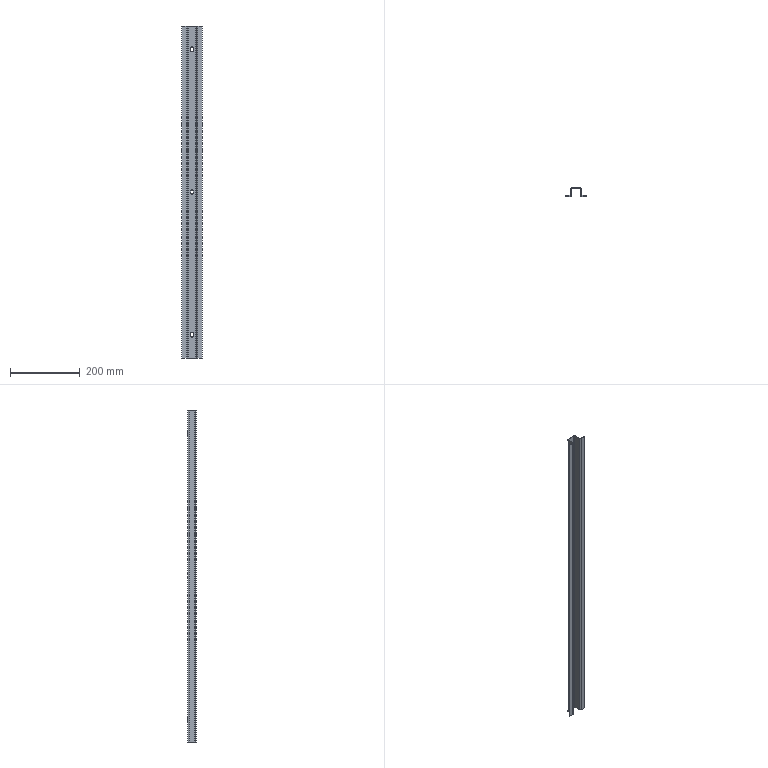Part | STEP file | B_SYL0380DJ1006_2_23-2_STEP | 1 solid | 56 faces | box 60 x 25 x 952 mm | volume 191493 mm3 | plane 36 | cylinder 20 | commonest cylinder face diameters 7 x12 4 x4 8 x4
STEP:
#1=CARTESIAN_POINT('',(-3.5,23.,-405.5));
#2=VERTEX_POINT('',#1);
#3=CARTESIAN_POINT('',(-3.5,25.,-405.5));
#4=VERTEX_POINT('',#3);
#5=CARTESIAN_POINT('',(-3.5,25.,-405.5));
#6=DIRECTION('',(0.,1.,0.));
#7=VECTOR('',#6,1000.);
#8=LINE('',#5,#7);
#9=EDGE_CURVE('',#2,#4,#8,.T.);
#10=ORIENTED_EDGE('',*,*,#9,.F.);
#11=CARTESIAN_POINT('',(-3.5,23.,-412.5));
#12=VERTEX_POINT('',#11);
#13=CARTESIAN_POINT('',(-3.5,23.,-476.));
#14=DIRECTION('',(0.,0.,1.));
#15=VECTOR('',#14,1000.);
#16=LINE('',#13,#15);
#17=EDGE_CURVE('',#12,#2,#16,.T.);
#18=ORIENTED_EDGE('',*,*,#17,.F.);
#19=CARTESIAN_POINT('',(-3.5,25.,-412.5));
#20=VERTEX_POINT('',#19);
#21=CARTESIAN_POINT('',(-3.5,25.,-412.5));
#22=DIRECTION('',(0.,1.,0.));
#23=VECTOR('',#22,1000.);
#24=LINE('',#21,#23);
#25=EDGE_CURVE('',#12,#20,#24,.T.);
#26=ORIENTED_EDGE('',*,*,#25,.T.);
#27=CARTESIAN_POINT('',(-3.5,25.,-412.5));
#28=DIRECTION('',(0.,0.,1.));
#29=VECTOR('',#28,1000.);
#30=LINE('',#27,#29);
#31=EDGE_CURVE('',#20,#4,#30,.T.);
#32=ORIENTED_EDGE('',*,*,#31,.T.);
#33=EDGE_LOOP('',(#10,#18,#26,#32));
#34=FACE_OUTER_BOUND('',#33,.T.);
#35=CARTESIAN_POINT('',(-3.5,25.,-412.5));
#36=DIRECTION('',(1.,0.,0.));
#37=DIRECTION('',(0.,0.,1.));
#38=AXIS2_PLACEMENT_3D('',#35,#36,#37);
#39=PLANE('',#38);
#40=ADVANCED_FACE('',(#34),#39,.T.);
#41=ORIENTED_EDGE('',*,*,#25,.F.);
#42=CARTESIAN_POINT('',(0.,23.,-416.));
#43=VERTEX_POINT('',#42);
#44=CARTESIAN_POINT('',(0.,23.,-412.5));
#45=DIRECTION('',(0.,-1.,0.));
#46=DIRECTION('',(0.,0.,-1.));
#47=AXIS2_PLACEMENT_3D('',#44,#45,#46);
#48=CIRCLE('',#47,3.5);
#49=EDGE_CURVE('',#12,#43,#48,.T.);
#50=ORIENTED_EDGE('',*,*,#49,.T.);
#51=CARTESIAN_POINT('',(0.,25.,-416.));
#52=VERTEX_POINT('',#51);
#53=CARTESIAN_POINT('',(0.,25.,-416.));
#54=DIRECTION('',(0.,1.,0.));
#55=VECTOR('',#54,1000.);
#56=LINE('',#53,#55);
#57=EDGE_CURVE('',#43,#52,#56,.T.);
#58=ORIENTED_EDGE('',*,*,#57,.T.);
#59=CARTESIAN_POINT('',(0.,25.,-412.5));
#60=DIRECTION('',(0.,-1.,0.));
#61=DIRECTION('',(-1.,0.,0.));
#62=AXIS2_PLACEMENT_3D('',#59,#60,#61);
#63=CIRCLE('',#62,3.5);
#64=EDGE_CURVE('',#20,#52,#63,.T.);
#65=ORIENTED_EDGE('',*,*,#64,.F.);
#66=EDGE_LOOP('',(#41,#50,#58,#65));
#67=FACE_OUTER_BOUND('',#66,.T.);
#68=CARTESIAN_POINT('',(0.,25.,-412.5));
#69=DIRECTION('',(0.,-1.,0.));
#70=DIRECTION('',(0.,0.,-1.));
#71=AXIS2_PLACEMENT_3D('',#68,#69,#70);
#72=CYLINDRICAL_SURFACE('',#71,3.5);
#73=ADVANCED_FACE('',(#67),#72,.F.);
#74=ORIENTED_EDGE('',*,*,#57,.F.);
#75=CARTESIAN_POINT('',(3.5,23.,-412.5));
#76=VERTEX_POINT('',#75);
#77=CARTESIAN_POINT('',(0.,23.,-412.5));
#78=DIRECTION('',(0.,-1.,0.));
#79=DIRECTION('',(0.,0.,-1.));
#80=AXIS2_PLACEMENT_3D('',#77,#78,#79);
#81=CIRCLE('',#80,3.5);
#82=EDGE_CURVE('',#43,#76,#81,.T.);
#83=ORIENTED_EDGE('',*,*,#82,.T.);
#84=CARTESIAN_POINT('',(3.5,25.,-412.5));
#85=VERTEX_POINT('',#84);
#86=CARTESIAN_POINT('',(3.5,25.,-412.5));
#87=DIRECTION('',(0.,1.,0.));
#88=VECTOR('',#87,1000.);
#89=LINE('',#86,#88);
#90=EDGE_CURVE('',#76,#85,#89,.T.);
#91=ORIENTED_EDGE('',*,*,#90,.T.);
#92=CARTESIAN_POINT('',(0.,25.,-412.5));
#93=DIRECTION('',(0.,-1.,0.));
#94=DIRECTION('',(0.,0.,-1.));
#95=AXIS2_PLACEMENT_3D('',#92,#93,#94);
#96=CIRCLE('',#95,3.5);
#97=EDGE_CURVE('',#52,#85,#96,.T.);
#98=ORIENTED_EDGE('',*,*,#97,.F.);
#99=EDGE_LOOP('',(#74,#83,#91,#98));
#100=FACE_OUTER_BOUND('',#99,.T.);
#101=CARTESIAN_POINT('',(0.,25.,-412.5));
#102=DIRECTION('',(0.,-1.,0.));
#103=DIRECTION('',(0.,0.,-1.));
#104=AXIS2_PLACEMENT_3D('',#101,#102,#103);
#105=CYLINDRICAL_SURFACE('',#104,3.5);
#106=ADVANCED_FACE('',(#100),#105,.F.);
#107=ORIENTED_EDGE('',*,*,#90,.F.);
#108=CARTESIAN_POINT('',(3.5,23.,-405.5));
#109=VERTEX_POINT('',#108);
#110=CARTESIAN_POINT('',(3.5,23.,-476.));
#111=DIRECTION('',(0.,0.,-1.));
#112=VECTOR('',#111,1000.);
#113=LINE('',#110,#112);
#114=EDGE_CURVE('',#109,#76,#113,.T.);
#115=ORIENTED_EDGE('',*,*,#114,.F.);
#116=CARTESIAN_POINT('',(3.5,25.,-405.5));
#117=VERTEX_POINT('',#116);
#118=CARTESIAN_POINT('',(3.5,25.,-405.5));
#119=DIRECTION('',(0.,1.,0.));
#120=VECTOR('',#119,1000.);
#121=LINE('',#118,#120);
#122=EDGE_CURVE('',#109,#117,#121,.T.);
#123=ORIENTED_EDGE('',*,*,#122,.T.);
#124=CARTESIAN_POINT('',(3.5,25.,-405.5));
#125=DIRECTION('',(0.,0.,-1.));
#126=VECTOR('',#125,1000.);
#127=LINE('',#124,#126);
#128=EDGE_CURVE('',#117,#85,#127,.T.);
#129=ORIENTED_EDGE('',*,*,#128,.T.);
#130=EDGE_LOOP('',(#107,#115,#123,#129));
#131=FACE_OUTER_BOUND('',#130,.T.);
#132=CARTESIAN_POINT('',(3.5,25.,-405.5));
#133=DIRECTION('',(-1.,0.,0.));
#134=DIRECTION('',(0.,0.,-1.));
#135=AXIS2_PLACEMENT_3D('',#132,#133,#134);
#136=PLANE('',#135);
#137=ADVANCED_FACE('',(#131),#136,.T.);
#138=ORIENTED_EDGE('',*,*,#122,.F.);
#139=CARTESIAN_POINT('',(0.,23.,-402.));
#140=VERTEX_POINT('',#139);
#141=CARTESIAN_POINT('',(0.,23.,-405.5));
#142=DIRECTION('',(0.,-1.,0.));
#143=DIRECTION('',(0.,0.,-1.));
#144=AXIS2_PLACEMENT_3D('',#141,#142,#143);
#145=CIRCLE('',#144,3.5);
#146=EDGE_CURVE('',#109,#140,#145,.T.);
#147=ORIENTED_EDGE('',*,*,#146,.T.);
#148=CARTESIAN_POINT('',(0.,25.,-402.));
#149=VERTEX_POINT('',#148);
#150=CARTESIAN_POINT('',(0.,25.,-402.));
#151=DIRECTION('',(0.,1.,0.));
#152=VECTOR('',#151,1000.);
#153=LINE('',#150,#152);
#154=EDGE_CURVE('',#140,#149,#153,.T.);
#155=ORIENTED_EDGE('',*,*,#154,.T.);
#156=CARTESIAN_POINT('',(0.,25.,-405.5));
#157=DIRECTION('',(0.,-1.,0.));
#158=DIRECTION('',(1.,0.,0.));
#159=AXIS2_PLACEMENT_3D('',#156,#157,#158);
#160=CIRCLE('',#159,3.5);
#161=EDGE_CURVE('',#117,#149,#160,.T.);
#162=ORIENTED_EDGE('',*,*,#161,.F.);
#163=EDGE_LOOP('',(#138,#147,#155,#162));
#164=FACE_OUTER_BOUND('',#163,.T.);
#165=CARTESIAN_POINT('',(0.,25.,-405.5));
#166=DIRECTION('',(0.,-1.,0.));
#167=DIRECTION('',(0.,0.,-1.));
#168=AXIS2_PLACEMENT_3D('',#165,#166,#167);
#169=CYLINDRICAL_SURFACE('',#168,3.5);
#170=ADVANCED_FACE('',(#164),#169,.F.);
#171=CARTESIAN_POINT('',(-3.5,23.,3.5));
#172=VERTEX_POINT('',#171);
#173=CARTESIAN_POINT('',(-3.5,25.,3.5));
#174=VERTEX_POINT('',#173);
#175=CARTESIAN_POINT('',(-3.5,25.,3.5));
#176=DIRECTION('',(0.,1.,0.));
#177=VECTOR('',#176,1000.);
#178=LINE('',#175,#177);
#179=EDGE_CURVE('',#172,#174,#178,.T.);
#180=ORIENTED_EDGE('',*,*,#179,.F.);
#181=CARTESIAN_POINT('',(-3.5,23.,-3.5));
#182=VERTEX_POINT('',#181);
#183=CARTESIAN_POINT('',(-3.5,23.,-476.));
#184=DIRECTION('',(0.,0.,1.));
#185=VECTOR('',#184,1000.);
#186=LINE('',#183,#185);
#187=EDGE_CURVE('',#182,#172,#186,.T.);
#188=ORIENTED_EDGE('',*,*,#187,.F.);
#189=CARTESIAN_POINT('',(-3.5,25.,-3.5));
#190=VERTEX_POINT('',#189);
#191=CARTESIAN_POINT('',(-3.5,25.,-3.5));
#192=DIRECTION('',(0.,1.,0.));
#193=VECTOR('',#192,1000.);
#194=LINE('',#191,#193);
#195=EDGE_CURVE('',#182,#190,#194,.T.);
#196=ORIENTED_EDGE('',*,*,#195,.T.);
#197=CARTESIAN_POINT('',(-3.5,25.,-3.5));
#198=DIRECTION('',(0.,0.,1.));
#199=VECTOR('',#198,1000.);
#200=LINE('',#197,#199);
#201=EDGE_CURVE('',#190,#174,#200,.T.);
#202=ORIENTED_EDGE('',*,*,#201,.T.);
#203=EDGE_LOOP('',(#180,#188,#196,#202));
#204=FACE_OUTER_BOUND('',#203,.T.);
#205=CARTESIAN_POINT('',(-3.5,25.,-3.5));
#206=DIRECTION('',(1.,0.,0.));
#207=DIRECTION('',(0.,0.,1.));
#208=AXIS2_PLACEMENT_3D('',#205,#206,#207);
#209=PLANE('',#208);
#210=ADVANCED_FACE('',(#204),#209,.T.);
#211=ORIENTED_EDGE('',*,*,#195,.F.);
#212=CARTESIAN_POINT('',(0.,23.,-7.));
#213=VERTEX_POINT('',#212);
#214=CARTESIAN_POINT('',(0.,23.,-3.5));
#215=DIRECTION('',(0.,-1.,0.));
#216=DIRECTION('',(0.,0.,-1.));
#217=AXIS2_PLACEMENT_3D('',#214,#215,#216);
#218=CIRCLE('',#217,3.5);
#219=EDGE_CURVE('',#182,#213,#218,.T.);
#220=ORIENTED_EDGE('',*,*,#219,.T.);
#221=CARTESIAN_POINT('',(0.,25.,-7.));
#222=VERTEX_POINT('',#221);
#223=CARTESIAN_POINT('',(0.,25.,-7.));
#224=DIRECTION('',(0.,1.,0.));
#225=VECTOR('',#224,1000.);
#226=LINE('',#223,#225);
#227=EDGE_CURVE('',#213,#222,#226,.T.);
#228=ORIENTED_EDGE('',*,*,#227,.T.);
#229=CARTESIAN_POINT('',(0.,25.,-3.5));
#230=DIRECTION('',(0.,-1.,0.));
#231=DIRECTION('',(-1.,0.,0.));
#232=AXIS2_PLACEMENT_3D('',#229,#230,#231);
#233=CIRCLE('',#232,3.5);
#234=EDGE_CURVE('',#190,#222,#233,.T.);
#235=ORIENTED_EDGE('',*,*,#234,.F.);
#236=EDGE_LOOP('',(#211,#220,#228,#235));
#237=FACE_OUTER_BOUND('',#236,.T.);
#238=CARTESIAN_POINT('',(0.,25.,-3.5));
#239=DIRECTION('',(0.,-1.,0.));
#240=DIRECTION('',(0.,0.,-1.));
#241=AXIS2_PLACEMENT_3D('',#238,#239,#240);
#242=CYLINDRICAL_SURFACE('',#241,3.5);
#243=ADVANCED_FACE('',(#237),#242,.F.);
#244=ORIENTED_EDGE('',*,*,#227,.F.);
#245=CARTESIAN_POINT('',(3.5,23.,-3.5));
#246=VERTEX_POINT('',#245);
#247=CARTESIAN_POINT('',(0.,23.,-3.5));
#248=DIRECTION('',(0.,-1.,0.));
#249=DIRECTION('',(0.,0.,-1.));
#250=AXIS2_PLACEMENT_3D('',#247,#248,#249);
#251=CIRCLE('',#250,3.5);
#252=EDGE_CURVE('',#213,#246,#251,.T.);
#253=ORIENTED_EDGE('',*,*,#252,.T.);
#254=CARTESIAN_POINT('',(3.5,25.,-3.5));
#255=VERTEX_POINT('',#254);
#256=CARTESIAN_POINT('',(3.5,25.,-3.5));
#257=DIRECTION('',(0.,1.,0.));
#258=VECTOR('',#257,1000.);
#259=LINE('',#256,#258);
#260=EDGE_CURVE('',#246,#255,#259,.T.);
#261=ORIENTED_EDGE('',*,*,#260,.T.);
#262=CARTESIAN_POINT('',(0.,25.,-3.5));
#263=DIRECTION('',(0.,-1.,0.));
#264=DIRECTION('',(0.,0.,-1.));
#265=AXIS2_PLACEMENT_3D('',#262,#263,#264);
#266=CIRCLE('',#265,3.5);
#267=EDGE_CURVE('',#222,#255,#266,.T.);
#268=ORIENTED_EDGE('',*,*,#267,.F.);
#269=EDGE_LOOP('',(#244,#253,#261,#268));
#270=FACE_OUTER_BOUND('',#269,.T.);
#271=CARTESIAN_POINT('',(0.,25.,-3.5));
#272=DIRECTION('',(0.,-1.,0.));
#273=DIRECTION('',(0.,0.,-1.));
#274=AXIS2_PLACEMENT_3D('',#271,#272,#273);
#275=CYLINDRICAL_SURFACE('',#274,3.5);
#276=ADVANCED_FACE('',(#270),#275,.F.);
#277=ORIENTED_EDGE('',*,*,#260,.F.);
#278=CARTESIAN_POINT('',(3.5,23.,3.5));
#279=VERTEX_POINT('',#278);
#280=CARTESIAN_POINT('',(3.5,23.,-476.));
#281=DIRECTION('',(0.,0.,-1.));
#282=VECTOR('',#281,1000.);
#283=LINE('',#280,#282);
#284=EDGE_CURVE('',#279,#246,#283,.T.);
#285=ORIENTED_EDGE('',*,*,#284,.F.);
#286=CARTESIAN_POINT('',(3.5,25.,3.5));
#287=VERTEX_POINT('',#286);
#288=CARTESIAN_POINT('',(3.5,25.,3.5));
#289=DIRECTION('',(0.,1.,0.));
#290=VECTOR('',#289,1000.);
#291=LINE('',#288,#290);
#292=EDGE_CURVE('',#279,#287,#291,.T.);
#293=ORIENTED_EDGE('',*,*,#292,.T.);
#294=CARTESIAN_POINT('',(3.5,25.,3.5));
#295=DIRECTION('',(0.,0.,-1.));
#296=VECTOR('',#295,1000.);
#297=LINE('',#294,#296);
#298=EDGE_CURVE('',#287,#255,#297,.T.);
#299=ORIENTED_EDGE('',*,*,#298,.T.);
#300=EDGE_LOOP('',(#277,#285,#293,#299));
#301=FACE_OUTER_BOUND('',#300,.T.);
#302=CARTESIAN_POINT('',(3.5,25.,3.5));
#303=DIRECTION('',(-1.,0.,0.));
#304=DIRECTION('',(0.,0.,-1.));
#305=AXIS2_PLACEMENT_3D('',#302,#303,#304);
#306=PLANE('',#305);
#307=ADVANCED_FACE('',(#301),#306,.T.);
#308=ORIENTED_EDGE('',*,*,#292,.F.);
#309=CARTESIAN_POINT('',(0.,23.,7.));
#310=VERTEX_POINT('',#309);
#311=CARTESIAN_POINT('',(0.,23.,3.5));
#312=DIRECTION('',(0.,-1.,0.));
#313=DIRECTION('',(0.,0.,-1.));
#314=AXIS2_PLACEMENT_3D('',#311,#312,#313);
#315=CIRCLE('',#314,3.5);
#316=EDGE_CURVE('',#279,#310,#315,.T.);
#317=ORIENTED_EDGE('',*,*,#316,.T.);
#318=CARTESIAN_POINT('',(0.,25.,7.));
#319=VERTEX_POINT('',#318);
#320=CARTESIAN_POINT('',(0.,25.,7.));
#321=DIRECTION('',(0.,1.,0.));
#322=VECTOR('',#321,1000.);
#323=LINE('',#320,#322);
#324=EDGE_CURVE('',#310,#319,#323,.T.);
#325=ORIENTED_EDGE('',*,*,#324,.T.);
#326=CARTESIAN_POINT('',(0.,25.,3.5));
#327=DIRECTION('',(0.,-1.,0.));
#328=DIRECTION('',(1.,0.,0.));
#329=AXIS2_PLACEMENT_3D('',#326,#327,#328);
#330=CIRCLE('',#329,3.5);
#331=EDGE_CURVE('',#287,#319,#330,.T.);
#332=ORIENTED_EDGE('',*,*,#331,.F.);
#333=EDGE_LOOP('',(#308,#317,#325,#332));
#334=FACE_OUTER_BOUND('',#333,.T.);
#335=CARTESIAN_POINT('',(0.,25.,3.5));
#336=DIRECTION('',(0.,-1.,0.));
#337=DIRECTION('',(0.,0.,-1.));
#338=AXIS2_PLACEMENT_3D('',#335,#336,#337);
#339=CYLINDRICAL_SURFACE('',#338,3.5);
#340=ADVANCED_FACE('',(#334),#339,.F.);
#341=CARTESIAN_POINT('',(-3.5,23.,412.5));
#342=VERTEX_POINT('',#341);
#343=CARTESIAN_POINT('',(-3.5,25.,412.5));
#344=VERTEX_POINT('',#343);
#345=CARTESIAN_POINT('',(-3.5,25.,412.5));
#346=DIRECTION('',(0.,1.,0.));
#347=VECTOR('',#346,1000.);
#348=LINE('',#345,#347);
#349=EDGE_CURVE('',#342,#344,#348,.T.);
#350=ORIENTED_EDGE('',*,*,#349,.F.);
#351=CARTESIAN_POINT('',(-3.5,23.,405.5));
#352=VERTEX_POINT('',#351);
#353=CARTESIAN_POINT('',(-3.5,23.,-476.));
#354=DIRECTION('',(0.,0.,1.));
#355=VECTOR('',#354,1000.);
#356=LINE('',#353,#355);
#357=EDGE_CURVE('',#352,#342,#356,.T.);
#358=ORIENTED_EDGE('',*,*,#357,.F.);
#359=CARTESIAN_POINT('',(-3.5,25.,405.5));
#360=VERTEX_POINT('',#359);
#361=CARTESIAN_POINT('',(-3.5,25.,405.5));
#362=DIRECTION('',(0.,1.,0.));
#363=VECTOR('',#362,1000.);
#364=LINE('',#361,#363);
#365=EDGE_CURVE('',#352,#360,#364,.T.);
#366=ORIENTED_EDGE('',*,*,#365,.T.);
#367=CARTESIAN_POINT('',(-3.5,25.,405.5));
#368=DIRECTION('',(0.,0.,1.));
#369=VECTOR('',#368,1000.);
#370=LINE('',#367,#369);
#371=EDGE_CURVE('',#360,#344,#370,.T.);
#372=ORIENTED_EDGE('',*,*,#371,.T.);
#373=EDGE_LOOP('',(#350,#358,#366,#372));
#374=FACE_OUTER_BOUND('',#373,.T.);
#375=CARTESIAN_POINT('',(-3.5,25.,405.5));
#376=DIRECTION('',(1.,0.,0.));
#377=DIRECTION('',(0.,0.,1.));
#378=AXIS2_PLACEMENT_3D('',#375,#376,#377);
#379=PLANE('',#378);
#380=ADVANCED_FACE('',(#374),#379,.T.);
#381=ORIENTED_EDGE('',*,*,#365,.F.);
#382=CARTESIAN_POINT('',(0.,23.,402.));
#383=VERTEX_POINT('',#382);
#384=CARTESIAN_POINT('',(0.,23.,405.5));
#385=DIRECTION('',(0.,-1.,0.));
#386=DIRECTION('',(0.,0.,-1.));
#387=AXIS2_PLACEMENT_3D('',#384,#385,#386);
#388=CIRCLE('',#387,3.5);
#389=EDGE_CURVE('',#352,#383,#388,.T.);
#390=ORIENTED_EDGE('',*,*,#389,.T.);
#391=CARTESIAN_POINT('',(0.,25.,402.));
#392=VERTEX_POINT('',#391);
#393=CARTESIAN_POINT('',(0.,25.,402.));
#394=DIRECTION('',(0.,1.,0.));
#395=VECTOR('',#394,1000.);
#396=LINE('',#393,#395);
#397=EDGE_CURVE('',#383,#392,#396,.T.);
#398=ORIENTED_EDGE('',*,*,#397,.T.);
#399=CARTESIAN_POINT('',(0.,25.,405.5));
#400=DIRECTION('',(0.,-1.,0.));
#401=DIRECTION('',(-1.,0.,0.));
#402=AXIS2_PLACEMENT_3D('',#399,#400,#401);
#403=CIRCLE('',#402,3.5);
#404=EDGE_CURVE('',#360,#392,#403,.T.);
#405=ORIENTED_EDGE('',*,*,#404,.F.);
#406=EDGE_LOOP('',(#381,#390,#398,#405));
#407=FACE_OUTER_BOUND('',#406,.T.);
#408=CARTESIAN_POINT('',(0.,25.,405.5));
#409=DIRECTION('',(0.,-1.,0.));
#410=DIRECTION('',(0.,0.,-1.));
#411=AXIS2_PLACEMENT_3D('',#408,#409,#410);
#412=CYLINDRICAL_SURFACE('',#411,3.5);
#413=ADVANCED_FACE('',(#407),#412,.F.);
#414=ORIENTED_EDGE('',*,*,#397,.F.);
#415=CARTESIAN_POINT('',(3.5,23.,405.5));
#416=VERTEX_POINT('',#415);
#417=CARTESIAN_POINT('',(0.,23.,405.5));
#418=DIRECTION('',(0.,-1.,0.));
#419=DIRECTION('',(0.,0.,-1.));
#420=AXIS2_PLACEMENT_3D('',#417,#418,#419);
#421=CIRCLE('',#420,3.5);
#422=EDGE_CURVE('',#383,#416,#421,.T.);
#423=ORIENTED_EDGE('',*,*,#422,.T.);
#424=CARTESIAN_POINT('',(3.5,25.,405.5));
#425=VERTEX_POINT('',#424);
#426=CARTESIAN_POINT('',(3.5,25.,405.5));
#427=DIRECTION('',(0.,1.,0.));
#428=VECTOR('',#427,1000.);
#429=LINE('',#426,#428);
#430=EDGE_CURVE('',#416,#425,#429,.T.);
#431=ORIENTED_EDGE('',*,*,#430,.T.);
#432=CARTESIAN_POINT('',(0.,25.,405.5));
#433=DIRECTION('',(0.,-1.,0.));
#434=DIRECTION('',(0.,0.,-1.));
#435=AXIS2_PLACEMENT_3D('',#432,#433,#434);
#436=CIRCLE('',#435,3.5);
#437=EDGE_CURVE('',#392,#425,#436,.T.);
#438=ORIENTED_EDGE('',*,*,#437,.F.);
#439=EDGE_LOOP('',(#414,#423,#431,#438));
#440=FACE_OUTER_BOUND('',#439,.T.);
#441=CARTESIAN_POINT('',(0.,25.,405.5));
#442=DIRECTION('',(0.,-1.,0.));
#443=DIRECTION('',(0.,0.,-1.));
#444=AXIS2_PLACEMENT_3D('',#441,#442,#443);
#445=CYLINDRICAL_SURFACE('',#444,3.5);
#446=ADVANCED_FACE('',(#440),#445,.F.);
#447=ORIENTED_EDGE('',*,*,#430,.F.);
#448=CARTESIAN_POINT('',(3.5,23.,412.5));
#449=VERTEX_POINT('',#448);
#450=CARTESIAN_POINT('',(3.5,23.,-476.));
#451=DIRECTION('',(0.,0.,-1.));
#452=VECTOR('',#451,1000.);
#453=LINE('',#450,#452);
#454=EDGE_CURVE('',#449,#416,#453,.T.);
#455=ORIENTED_EDGE('',*,*,#454,.F.);
#456=CARTESIAN_POINT('',(3.5,25.,412.5));
#457=VERTEX_POINT('',#456);
#458=CARTESIAN_POINT('',(3.5,25.,412.5));
#459=DIRECTION('',(0.,1.,0.));
#460=VECTOR('',#459,1000.);
#461=LINE('',#458,#460);
#462=EDGE_CURVE('',#449,#457,#461,.T.);
#463=ORIENTED_EDGE('',*,*,#462,.T.);
#464=CARTESIAN_POINT('',(3.5,25.,412.5));
#465=DIRECTION('',(0.,0.,-1.));
#466=VECTOR('',#465,1000.);
#467=LINE('',#464,#466);
#468=EDGE_CURVE('',#457,#425,#467,.T.);
#469=ORIENTED_EDGE('',*,*,#468,.T.);
#470=EDGE_LOOP('',(#447,#455,#463,#469));
#471=FACE_OUTER_BOUND('',#470,.T.);
#472=CARTESIAN_POINT('',(3.5,25.,412.5));
#473=DIRECTION('',(-1.,0.,0.));
#474=DIRECTION('',(0.,0.,-1.));
#475=AXIS2_PLACEMENT_3D('',#472,#473,#474);
#476=PLANE('',#475);
#477=ADVANCED_FACE('',(#471),#476,.T.);
#478=ORIENTED_EDGE('',*,*,#462,.F.);
#479=CARTESIAN_POINT('',(0.,23.,416.));
#480=VERTEX_POINT('',#479);
#481=CARTESIAN_POINT('',(0.,23.,412.5));
#482=DIRECTION('',(0.,-1.,0.));
#483=DIRECTION('',(0.,0.,-1.));
#484=AXIS2_PLACEMENT_3D('',#481,#482,#483);
#485=CIRCLE('',#484,3.5);
#486=EDGE_CURVE('',#449,#480,#485,.T.);
#487=ORIENTED_EDGE('',*,*,#486,.T.);
#488=CARTESIAN_POINT('',(0.,25.,416.));
#489=VERTEX_POINT('',#488);
#490=CARTESIAN_POINT('',(0.,25.,416.));
#491=DIRECTION('',(0.,1.,0.));
#492=VECTOR('',#491,1000.);
#493=LINE('',#490,#492);
#494=EDGE_CURVE('',#480,#489,#493,.T.);
#495=ORIENTED_EDGE('',*,*,#494,.T.);
#496=CARTESIAN_POINT('',(0.,25.,412.5));
#497=DIRECTION('',(0.,-1.,0.));
#498=DIRECTION('',(1.,0.,0.));
#499=AXIS2_PLACEMENT_3D('',#496,#497,#498);
#500=CIRCLE('',#499,3.5);
#501=EDGE_CURVE('',#457,#489,#500,.T.);
#502=ORIENTED_EDGE('',*,*,#501,.F.);
#503=EDGE_LOOP('',(#478,#487,#495,#502));
#504=FACE_OUTER_BOUND('',#503,.T.);
#505=CARTESIAN_POINT('',(0.,25.,412.5));
#506=DIRECTION('',(0.,-1.,0.));
#507=DIRECTION('',(0.,0.,-1.));
#508=AXIS2_PLACEMENT_3D('',#505,#506,#507);
#509=CYLINDRICAL_SURFACE('',#508,3.5);
#510=ADVANCED_FACE('',(#504),#509,.F.);
#511=CARTESIAN_POINT('',(-30.,0.,-476.));
#512=VERTEX_POINT('',#511);
#513=CARTESIAN_POINT('',(-30.,2.,-476.));
#514=VERTEX_POINT('',#513);
#515=CARTESIAN_POINT('',(-30.,2.,-476.));
#516=DIRECTION('',(0.,1.,0.));
#517=VECTOR('',#516,1000.);
#518=LINE('',#515,#517);
#519=EDGE_CURVE('',#512,#514,#518,.T.);
#520=ORIENTED_EDGE('',*,*,#519,.F.);
#521=CARTESIAN_POINT('',(-30.,0.,476.));
#522=VERTEX_POINT('',#521);
#523=CARTESIAN_POINT('',(-30.,0.,-476.));
#524=DIRECTION('',(0.,0.,-1.));
#525=VECTOR('',#524,1000.);
#526=LINE('',#523,#525);
#527=EDGE_CURVE('',#522,#512,#526,.T.);
#528=ORIENTED_EDGE('',*,*,#527,.F.);
#529=CARTESIAN_POINT('',(-30.,2.,476.));
#530=VERTEX_POINT('',#529);
#531=CARTESIAN_POINT('',(-30.,2.,476.));
#532=DIRECTION('',(0.,1.,0.));
#533=VECTOR('',#532,1000.);
#534=LINE('',#531,#533);
#535=EDGE_CURVE('',#522,#530,#534,.T.);
#536=ORIENTED_EDGE('',*,*,#535,.T.);
#537=CARTESIAN_POINT('',(-30.,2.,476.));
#538=DIRECTION('',(0.,0.,-1.));
#539=VECTOR('',#538,1000.);
#540=LINE('',#537,#539);
#541=EDGE_CURVE('',#530,#514,#540,.T.);
#542=ORIENTED_EDGE('',*,*,#541,.T.);
#543=EDGE_LOOP('',(#520,#528,#536,#542));
#544=FACE_OUTER_BOUND('',#543,.T.);
#545=CARTESIAN_POINT('',(-30.,2.,476.));
#546=DIRECTION('',(-1.,0.,0.));
#547=DIRECTION('',(0.,0.,-1.));
#548=AXIS2_PLACEMENT_3D('',#545,#546,#547);
#549=PLANE('',#548);
#550=ADVANCED_FACE('',(#544),#549,.T.);
#551=ORIENTED_EDGE('',*,*,#535,.F.);
#552=CARTESIAN_POINT('',(-17.,0.,476.));
#553=VERTEX_POINT('',#552);
#554=CARTESIAN_POINT('',(-30.,0.,476.));
#555=DIRECTION('',(-1.,0.,0.));
#556=VECTOR('',#555,1000.);
#557=LINE('',#554,#556);
#558=EDGE_CURVE('',#553,#522,#557,.T.);
#559=ORIENTED_EDGE('',*,*,#558,.F.);
#560=CARTESIAN_POINT('',(-17.,2.,476.));
#561=VERTEX_POINT('',#560);
#562=CARTESIAN_POINT('',(-17.,2.,476.));
#563=DIRECTION('',(0.,1.,0.));
#564=VECTOR('',#563,1000.);
#565=LINE('',#562,#564);
#566=EDGE_CURVE('',#553,#561,#565,.T.);
#567=ORIENTED_EDGE('',*,*,#566,.T.);
#568=CARTESIAN_POINT('',(-17.,2.,476.));
#569=DIRECTION('',(-1.,0.,0.));
#570=VECTOR('',#569,1000.);
#571=LINE('',#568,#570);
#572=EDGE_CURVE('',#561,#530,#571,.T.);
#573=ORIENTED_EDGE('',*,*,#572,.T.);
#574=EDGE_LOOP('',(#551,#559,#567,#573));
#575=FACE_OUTER_BOUND('',#574,.T.);
#576=CARTESIAN_POINT('',(-17.,2.,476.));
#577=DIRECTION('',(0.,0.,1.));
#578=DIRECTION('',(-1.,0.,0.));
#579=AXIS2_PLACEMENT_3D('',#576,#577,#578);
#580=PLANE('',#579);
#581=ADVANCED_FACE('',(#575),#580,.T.);
#582=ORIENTED_EDGE('',*,*,#566,.F.);
#583=CARTESIAN_POINT('',(-13.,4.,476.));
#584=VERTEX_POINT('',#583);
#585=CARTESIAN_POINT('',(-17.,4.,476.));
#586=DIRECTION('',(0.,0.,-1.));
#587=DIRECTION('',(1.,0.,0.));
#588=AXIS2_PLACEMENT_3D('',#585,#586,#587);
#589=CIRCLE('',#588,4.);
#590=EDGE_CURVE('',#584,#553,#589,.T.);
#591=ORIENTED_EDGE('',*,*,#590,.F.);
#592=CARTESIAN_POINT('',(-15.,4.,476.));
#593=VERTEX_POINT('',#592);
#594=CARTESIAN_POINT('',(-15.,4.,476.));
#595=DIRECTION('',(-1.,0.,0.));
#596=VECTOR('',#595,1000.);
#597=LINE('',#594,#596);
#598=EDGE_CURVE('',#584,#593,#597,.T.);
#599=ORIENTED_EDGE('',*,*,#598,.T.);
#600=CARTESIAN_POINT('',(-17.,4.,476.));
#601=DIRECTION('',(0.,0.,-1.));
#602=DIRECTION('',(1.,0.,0.));
#603=AXIS2_PLACEMENT_3D('',#600,#601,#602);
#604=CIRCLE('',#603,2.);
#605=EDGE_CURVE('',#593,#561,#604,.T.);
#606=ORIENTED_EDGE('',*,*,#605,.T.);
#607=EDGE_LOOP('',(#582,#591,#599,#606));
#608=FACE_OUTER_BOUND('',#607,.T.);
#609=CARTESIAN_POINT('',(-17.,4.,476.));
#610=DIRECTION('',(0.,0.,1.));
#611=DIRECTION('',(1.,0.,0.));
#612=AXIS2_PLACEMENT_3D('',#609,#610,#611);
#613=PLANE('',#612);
#614=ADVANCED_FACE('',(#608),#613,.T.);
#615=ORIENTED_EDGE('',*,*,#598,.F.);
#616=CARTESIAN_POINT('',(-13.,21.,476.));
#617=VERTEX_POINT('',#616);
#618=CARTESIAN_POINT('',(-13.,4.,476.));
#619=DIRECTION('',(0.,-1.,0.));
#620=VECTOR('',#619,1000.);
#621=LINE('',#618,#620);
#622=EDGE_CURVE('',#617,#584,#621,.T.);
#623=ORIENTED_EDGE('',*,*,#622,.F.);
#624=CARTESIAN_POINT('',(-15.,21.,476.));
#625=VERTEX_POINT('',#624);
#626=CARTESIAN_POINT('',(-15.,21.,476.));
#627=DIRECTION('',(-1.,0.,0.));
#628=VECTOR('',#627,1000.);
#629=LINE('',#626,#628);
#630=EDGE_CURVE('',#617,#625,#629,.T.);
#631=ORIENTED_EDGE('',*,*,#630,.T.);
#632=CARTESIAN_POINT('',(-15.,21.,476.));
#633=DIRECTION('',(0.,-1.,0.));
#634=VECTOR('',#633,1000.);
#635=LINE('',#632,#634);
#636=EDGE_CURVE('',#625,#593,#635,.T.);
#637=ORIENTED_EDGE('',*,*,#636,.T.);
#638=EDGE_LOOP('',(#615,#623,#631,#637));
#639=FACE_OUTER_BOUND('',#638,.T.);
#640=CARTESIAN_POINT('',(-15.,21.,476.));
#641=DIRECTION('',(0.,0.,1.));
#642=DIRECTION('',(0.,-1.,0.));
#643=AXIS2_PLACEMENT_3D('',#640,#641,#642);
#644=PLANE('',#643);
#645=ADVANCED_FACE('',(#639),#644,.T.);
#646=ORIENTED_EDGE('',*,*,#630,.F.);
#647=CARTESIAN_POINT('',(-11.,23.,476.));
#648=VERTEX_POINT('',#647);
#649=CARTESIAN_POINT('',(-11.,21.,476.));
#650=DIRECTION('',(0.,0.,1.));
#651=DIRECTION('',(1.,0.,0.));
#652=AXIS2_PLACEMENT_3D('',#649,#650,#651);
#653=CIRCLE('',#652,2.);
#654=EDGE_CURVE('',#648,#617,#653,.T.);
#655=ORIENTED_EDGE('',*,*,#654,.F.);
#656=CARTESIAN_POINT('',(-11.,25.,476.));
#657=VERTEX_POINT('',#656);
#658=CARTESIAN_POINT('',(-11.,25.,476.));
#659=DIRECTION('',(0.,1.,0.));
#660=VECTOR('',#659,1000.);
#661=LINE('',#658,#660);
#662=EDGE_CURVE('',#648,#657,#661,.T.);
#663=ORIENTED_EDGE('',*,*,#662,.T.);
#664=CARTESIAN_POINT('',(-11.,21.,476.));
#665=DIRECTION('',(0.,0.,1.));
#666=DIRECTION('',(0.,1.,0.));
#667=AXIS2_PLACEMENT_3D('',#664,#665,#666);
#668=CIRCLE('',#667,4.);
#669=EDGE_CURVE('',#657,#625,#668,.T.);
#670=ORIENTED_EDGE('',*,*,#669,.T.);
#671=EDGE_LOOP('',(#646,#655,#663,#670));
#672=FACE_OUTER_BOUND('',#671,.T.);
#673=CARTESIAN_POINT('',(-11.,21.,476.));
#674=DIRECTION('',(0.,0.,-1.));
#675=DIRECTION('',(-1.,0.,0.));
#676=AXIS2_PLACEMENT_3D('',#673,#674,#675);
#677=PLANE('',#676);
#678=ADVANCED_FACE('',(#672),#677,.F.);
#679=ORIENTED_EDGE('',*,*,#662,.F.);
#680=CARTESIAN_POINT('',(11.,23.,476.));
#681=VERTEX_POINT('',#680);
#682=CARTESIAN_POINT('',(-11.,23.,476.));
#683=DIRECTION('',(-1.,0.,0.));
#684=VECTOR('',#683,1000.);
#685=LINE('',#682,#684);
#686=EDGE_CURVE('',#681,#648,#685,.T.);
#687=ORIENTED_EDGE('',*,*,#686,.F.);
#688=CARTESIAN_POINT('',(11.,25.,476.));
#689=VERTEX_POINT('',#688);
#690=CARTESIAN_POINT('',(11.,25.,476.));
#691=DIRECTION('',(0.,1.,0.));
#692=VECTOR('',#691,1000.);
#693=LINE('',#690,#692);
#694=EDGE_CURVE('',#681,#689,#693,.T.);
#695=ORIENTED_EDGE('',*,*,#694,.T.);
#696=CARTESIAN_POINT('',(11.,25.,476.));
#697=DIRECTION('',(-1.,0.,0.));
#698=VECTOR('',#697,1000.);
#699=LINE('',#696,#698);
#700=EDGE_CURVE('',#689,#657,#699,.T.);
#701=ORIENTED_EDGE('',*,*,#700,.T.);
#702=EDGE_LOOP('',(#679,#687,#695,#701));
#703=FACE_OUTER_BOUND('',#702,.T.);
#704=CARTESIAN_POINT('',(11.,25.,476.));
#705=DIRECTION('',(0.,0.,1.));
#706=DIRECTION('',(-1.,0.,0.));
#707=AXIS2_PLACEMENT_3D('',#704,#705,#706);
#708=PLANE('',#707);
#709=ADVANCED_FACE('',(#703),#708,.T.);
#710=ORIENTED_EDGE('',*,*,#694,.F.);
#711=CARTESIAN_POINT('',(13.,21.,476.));
#712=VERTEX_POINT('',#711);
#713=CARTESIAN_POINT('',(11.,21.,476.));
#714=DIRECTION('',(0.,0.,1.));
#715=DIRECTION('',(1.,0.,0.));
#716=AXIS2_PLACEMENT_3D('',#713,#714,#715);
#717=CIRCLE('',#716,2.);
#718=EDGE_CURVE('',#712,#681,#717,.T.);
#719=ORIENTED_EDGE('',*,*,#718,.F.);
#720=CARTESIAN_POINT('',(15.,21.,476.));
#721=VERTEX_POINT('',#720);
#722=CARTESIAN_POINT('',(15.,21.,476.));
#723=DIRECTION('',(1.,0.,0.));
#724=VECTOR('',#723,1000.);
#725=LINE('',#722,#724);
#726=EDGE_CURVE('',#712,#721,#725,.T.);
#727=ORIENTED_EDGE('',*,*,#726,.T.);
#728=CARTESIAN_POINT('',(11.,21.,476.));
#729=DIRECTION('',(0.,0.,1.));
#730=DIRECTION('',(1.,0.,0.));
#731=AXIS2_PLACEMENT_3D('',#728,#729,#730);
#732=CIRCLE('',#731,4.);
#733=EDGE_CURVE('',#721,#689,#732,.T.);
#734=ORIENTED_EDGE('',*,*,#733,.T.);
#735=EDGE_LOOP('',(#710,#719,#727,#734));
#736=FACE_OUTER_BOUND('',#735,.T.);
#737=CARTESIAN_POINT('',(11.,21.,476.));
#738=DIRECTION('',(0.,0.,-1.));
#739=DIRECTION('',(-1.,0.,0.));
#740=AXIS2_PLACEMENT_3D('',#737,#738,#739);
#741=PLANE('',#740);
#742=ADVANCED_FACE('',(#736),#741,.F.);
#743=ORIENTED_EDGE('',*,*,#726,.F.);
#744=CARTESIAN_POINT('',(13.,4.,476.));
#745=VERTEX_POINT('',#744);
#746=CARTESIAN_POINT('',(13.,21.,476.));
#747=DIRECTION('',(0.,1.,0.));
#748=VECTOR('',#747,1000.);
#749=LINE('',#746,#748);
#750=EDGE_CURVE('',#745,#712,#749,.T.);
#751=ORIENTED_EDGE('',*,*,#750,.F.);
#752=CARTESIAN_POINT('',(15.,4.,476.));
#753=VERTEX_POINT('',#752);
#754=CARTESIAN_POINT('',(15.,4.,476.));
#755=DIRECTION('',(1.,0.,0.));
#756=VECTOR('',#755,1000.);
#757=LINE('',#754,#756);
#758=EDGE_CURVE('',#745,#753,#757,.T.);
#759=ORIENTED_EDGE('',*,*,#758,.T.);
#760=CARTESIAN_POINT('',(15.,4.,476.));
#761=DIRECTION('',(0.,1.,0.));
#762=VECTOR('',#761,1000.);
#763=LINE('',#760,#762);
#764=EDGE_CURVE('',#753,#721,#763,.T.);
#765=ORIENTED_EDGE('',*,*,#764,.T.);
#766=EDGE_LOOP('',(#743,#751,#759,#765));
#767=FACE_OUTER_BOUND('',#766,.T.);
#768=CARTESIAN_POINT('',(15.,4.,476.));
#769=DIRECTION('',(0.,0.,1.));
#770=DIRECTION('',(0.,1.,0.));
#771=AXIS2_PLACEMENT_3D('',#768,#769,#770);
#772=PLANE('',#771);
#773=ADVANCED_FACE('',(#767),#772,.T.);
#774=ORIENTED_EDGE('',*,*,#758,.F.);
#775=CARTESIAN_POINT('',(17.,0.,476.));
#776=VERTEX_POINT('',#775);
#777=CARTESIAN_POINT('',(17.,4.,476.));
#778=DIRECTION('',(0.,0.,-1.));
#779=DIRECTION('',(1.,0.,0.));
#780=AXIS2_PLACEMENT_3D('',#777,#778,#779);
#781=CIRCLE('',#780,4.);
#782=EDGE_CURVE('',#776,#745,#781,.T.);
#783=ORIENTED_EDGE('',*,*,#782,.F.);
#784=CARTESIAN_POINT('',(17.,2.,476.));
#785=VERTEX_POINT('',#784);
#786=CARTESIAN_POINT('',(17.,2.,476.));
#787=DIRECTION('',(0.,1.,0.));
#788=VECTOR('',#787,1000.);
#789=LINE('',#786,#788);
#790=EDGE_CURVE('',#776,#785,#789,.T.);
#791=ORIENTED_EDGE('',*,*,#790,.T.);
#792=CARTESIAN_POINT('',(17.,4.,476.));
#793=DIRECTION('',(0.,0.,-1.));
#794=DIRECTION('',(0.,-1.,0.));
#795=AXIS2_PLACEMENT_3D('',#792,#793,#794);
#796=CIRCLE('',#795,2.);
#797=EDGE_CURVE('',#785,#753,#796,.T.);
#798=ORIENTED_EDGE('',*,*,#797,.T.);
#799=EDGE_LOOP('',(#774,#783,#791,#798));
#800=FACE_OUTER_BOUND('',#799,.T.);
#801=CARTESIAN_POINT('',(17.,4.,476.));
#802=DIRECTION('',(0.,0.,1.));
#803=DIRECTION('',(1.,0.,0.));
#804=AXIS2_PLACEMENT_3D('',#801,#802,#803);
#805=PLANE('',#804);
#806=ADVANCED_FACE('',(#800),#805,.T.);
#807=ORIENTED_EDGE('',*,*,#790,.F.);
#808=CARTESIAN_POINT('',(30.,0.,476.));
#809=VERTEX_POINT('',#808);
#810=CARTESIAN_POINT('',(17.,0.,476.));
#811=DIRECTION('',(-1.,0.,0.));
#812=VECTOR('',#811,1000.);
#813=LINE('',#810,#812);
#814=EDGE_CURVE('',#809,#776,#813,.T.);
#815=ORIENTED_EDGE('',*,*,#814,.F.);
#816=CARTESIAN_POINT('',(30.,2.,476.));
#817=VERTEX_POINT('',#816);
#818=CARTESIAN_POINT('',(30.,2.,476.));
#819=DIRECTION('',(0.,1.,0.));
#820=VECTOR('',#819,1000.);
#821=LINE('',#818,#820);
#822=EDGE_CURVE('',#809,#817,#821,.T.);
#823=ORIENTED_EDGE('',*,*,#822,.T.);
#824=CARTESIAN_POINT('',(30.,2.,476.));
#825=DIRECTION('',(-1.,0.,0.));
#826=VECTOR('',#825,1000.);
#827=LINE('',#824,#826);
#828=EDGE_CURVE('',#817,#785,#827,.T.);
#829=ORIENTED_EDGE('',*,*,#828,.T.);
#830=EDGE_LOOP('',(#807,#815,#823,#829));
#831=FACE_OUTER_BOUND('',#830,.T.);
#832=CARTESIAN_POINT('',(30.,2.,476.));
#833=DIRECTION('',(0.,0.,1.));
#834=DIRECTION('',(-1.,0.,0.));
#835=AXIS2_PLACEMENT_3D('',#832,#833,#834);
#836=PLANE('',#835);
#837=ADVANCED_FACE('',(#831),#836,.T.);
#838=ORIENTED_EDGE('',*,*,#822,.F.);
#839=CARTESIAN_POINT('',(30.,0.,-476.));
#840=VERTEX_POINT('',#839);
#841=CARTESIAN_POINT('',(30.,0.,-476.));
#842=DIRECTION('',(0.,0.,-1.));
#843=VECTOR('',#842,1000.);
#844=LINE('',#841,#843);
#845=EDGE_CURVE('',#809,#840,#844,.T.);
#846=ORIENTED_EDGE('',*,*,#845,.T.);
#847=CARTESIAN_POINT('',(30.,2.,-476.));
#848=VERTEX_POINT('',#847);
#849=CARTESIAN_POINT('',(30.,2.,-476.));
#850=DIRECTION('',(0.,1.,0.));
#851=VECTOR('',#850,1000.);
#852=LINE('',#849,#851);
#853=EDGE_CURVE('',#840,#848,#852,.T.);
#854=ORIENTED_EDGE('',*,*,#853,.T.);
#855=CARTESIAN_POINT('',(30.,2.,476.));
#856=DIRECTION('',(0.,0.,-1.));
#857=VECTOR('',#856,1000.);
#858=LINE('',#855,#857);
#859=EDGE_CURVE('',#817,#848,#858,.T.);
#860=ORIENTED_EDGE('',*,*,#859,.F.);
#861=EDGE_LOOP('',(#838,#846,#854,#860));
#862=FACE_OUTER_BOUND('',#861,.T.);
#863=CARTESIAN_POINT('',(30.,2.,476.));
#864=DIRECTION('',(-1.,0.,0.));
#865=DIRECTION('',(0.,0.,-1.));
#866=AXIS2_PLACEMENT_3D('',#863,#864,#865);
#867=PLANE('',#866);
#868=ADVANCED_FACE('',(#862),#867,.F.);
#869=ORIENTED_EDGE('',*,*,#853,.F.);
#870=CARTESIAN_POINT('',(17.,0.,-476.));
#871=VERTEX_POINT('',#870);
#872=CARTESIAN_POINT('',(17.,0.,-476.));
#873=DIRECTION('',(-1.,0.,0.));
#874=VECTOR('',#873,1000.);
#875=LINE('',#872,#874);
#876=EDGE_CURVE('',#840,#871,#875,.T.);
#877=ORIENTED_EDGE('',*,*,#876,.T.);
#878=CARTESIAN_POINT('',(17.,2.,-476.));
#879=VERTEX_POINT('',#878);
#880=CARTESIAN_POINT('',(17.,2.,-476.));
#881=DIRECTION('',(0.,1.,0.));
#882=VECTOR('',#881,1000.);
#883=LINE('',#880,#882);
#884=EDGE_CURVE('',#871,#879,#883,.T.);
#885=ORIENTED_EDGE('',*,*,#884,.T.);
#886=CARTESIAN_POINT('',(30.,2.,-476.));
#887=DIRECTION('',(-1.,0.,0.));
#888=VECTOR('',#887,1000.);
#889=LINE('',#886,#888);
#890=EDGE_CURVE('',#848,#879,#889,.T.);
#891=ORIENTED_EDGE('',*,*,#890,.F.);
#892=EDGE_LOOP('',(#869,#877,#885,#891));
#893=FACE_OUTER_BOUND('',#892,.T.);
#894=CARTESIAN_POINT('',(30.,2.,-476.));
#895=DIRECTION('',(0.,0.,1.));
#896=DIRECTION('',(-1.,0.,0.));
#897=AXIS2_PLACEMENT_3D('',#894,#895,#896);
#898=PLANE('',#897);
#899=ADVANCED_FACE('',(#893),#898,.F.);
#900=ORIENTED_EDGE('',*,*,#884,.F.);
#901=CARTESIAN_POINT('',(13.,4.,-476.));
#902=VERTEX_POINT('',#901);
#903=CARTESIAN_POINT('',(17.,4.,-476.));
#904=DIRECTION('',(0.,0.,1.));
#905=DIRECTION('',(1.,0.,0.));
#906=AXIS2_PLACEMENT_3D('',#903,#904,#905);
#907=CIRCLE('',#906,4.);
#908=EDGE_CURVE('',#902,#871,#907,.T.);
#909=ORIENTED_EDGE('',*,*,#908,.F.);
#910=CARTESIAN_POINT('',(15.,4.,-476.));
#911=VERTEX_POINT('',#910);
#912=CARTESIAN_POINT('',(15.,4.,-476.));
#913=DIRECTION('',(1.,0.,0.));
#914=VECTOR('',#913,1000.);
#915=LINE('',#912,#914);
#916=EDGE_CURVE('',#902,#911,#915,.T.);
#917=ORIENTED_EDGE('',*,*,#916,.T.);
#918=CARTESIAN_POINT('',(17.,4.,-476.));
#919=DIRECTION('',(0.,0.,1.));
#920=DIRECTION('',(-1.,0.,0.));
#921=AXIS2_PLACEMENT_3D('',#918,#919,#920);
#922=CIRCLE('',#921,2.);
#923=EDGE_CURVE('',#911,#879,#922,.T.);
#924=ORIENTED_EDGE('',*,*,#923,.T.);
#925=EDGE_LOOP('',(#900,#909,#917,#924));
#926=FACE_OUTER_BOUND('',#925,.T.);
#927=CARTESIAN_POINT('',(17.,4.,-476.));
#928=DIRECTION('',(0.,0.,-1.));
#929=DIRECTION('',(-1.,0.,0.));
#930=AXIS2_PLACEMENT_3D('',#927,#928,#929);
#931=PLANE('',#930);
#932=ADVANCED_FACE('',(#926),#931,.T.);
#933=ORIENTED_EDGE('',*,*,#916,.F.);
#934=CARTESIAN_POINT('',(13.,21.,-476.));
#935=VERTEX_POINT('',#934);
#936=CARTESIAN_POINT('',(13.,21.,-476.));
#937=DIRECTION('',(0.,1.,0.));
#938=VECTOR('',#937,1000.);
#939=LINE('',#936,#938);
#940=EDGE_CURVE('',#902,#935,#939,.T.);
#941=ORIENTED_EDGE('',*,*,#940,.T.);
#942=CARTESIAN_POINT('',(15.,21.,-476.));
#943=VERTEX_POINT('',#942);
#944=CARTESIAN_POINT('',(15.,21.,-476.));
#945=DIRECTION('',(1.,0.,0.));
#946=VECTOR('',#945,1000.);
#947=LINE('',#944,#946);
#948=EDGE_CURVE('',#935,#943,#947,.T.);
#949=ORIENTED_EDGE('',*,*,#948,.T.);
#950=CARTESIAN_POINT('',(15.,4.,-476.));
#951=DIRECTION('',(0.,1.,0.));
#952=VECTOR('',#951,1000.);
#953=LINE('',#950,#952);
#954=EDGE_CURVE('',#911,#943,#953,.T.);
#955=ORIENTED_EDGE('',*,*,#954,.F.);
#956=EDGE_LOOP('',(#933,#941,#949,#955));
#957=FACE_OUTER_BOUND('',#956,.T.);
#958=CARTESIAN_POINT('',(15.,4.,-476.));
#959=DIRECTION('',(0.,0.,1.));
#960=DIRECTION('',(0.,1.,0.));
#961=AXIS2_PLACEMENT_3D('',#958,#959,#960);
#962=PLANE('',#961);
#963=ADVANCED_FACE('',(#957),#962,.F.);
#964=ORIENTED_EDGE('',*,*,#948,.F.);
#965=CARTESIAN_POINT('',(11.,23.,-476.));
#966=VERTEX_POINT('',#965);
#967=CARTESIAN_POINT('',(11.,21.,-476.));
#968=DIRECTION('',(0.,0.,-1.));
#969=DIRECTION('',(1.,0.,0.));
#970=AXIS2_PLACEMENT_3D('',#967,#968,#969);
#971=CIRCLE('',#970,2.);
#972=EDGE_CURVE('',#966,#935,#971,.T.);
#973=ORIENTED_EDGE('',*,*,#972,.F.);
#974=CARTESIAN_POINT('',(11.,25.,-476.));
#975=VERTEX_POINT('',#974);
#976=CARTESIAN_POINT('',(11.,25.,-476.));
#977=DIRECTION('',(0.,1.,0.));
#978=VECTOR('',#977,1000.);
#979=LINE('',#976,#978);
#980=EDGE_CURVE('',#966,#975,#979,.T.);
#981=ORIENTED_EDGE('',*,*,#980,.T.);
#982=CARTESIAN_POINT('',(11.,21.,-476.));
#983=DIRECTION('',(0.,0.,-1.));
#984=DIRECTION('',(0.,1.,0.));
#985=AXIS2_PLACEMENT_3D('',#982,#983,#984);
#986=CIRCLE('',#985,4.);
#987=EDGE_CURVE('',#975,#943,#986,.T.);
#988=ORIENTED_EDGE('',*,*,#987,.T.);
#989=EDGE_LOOP('',(#964,#973,#981,#988));
#990=FACE_OUTER_BOUND('',#989,.T.);
#991=CARTESIAN_POINT('',(11.,21.,-476.));
#992=DIRECTION('',(0.,0.,1.));
#993=DIRECTION('',(1.,0.,0.));
#994=AXIS2_PLACEMENT_3D('',#991,#992,#993);
#995=PLANE('',#994);
#996=ADVANCED_FACE('',(#990),#995,.F.);
#997=ORIENTED_EDGE('',*,*,#980,.F.);
#998=CARTESIAN_POINT('',(-11.,23.,-476.));
#999=VERTEX_POINT('',#998);
#1000=CARTESIAN_POINT('',(-11.,23.,-476.));
#1001=DIRECTION('',(-1.,0.,0.));
#1002=VECTOR('',#1001,1000.);
#1003=LINE('',#1000,#1002);
#1004=EDGE_CURVE('',#966,#999,#1003,.T.);
#1005=ORIENTED_EDGE('',*,*,#1004,.T.);
#1006=CARTESIAN_POINT('',(-11.,25.,-476.));
#1007=VERTEX_POINT('',#1006);
#1008=CARTESIAN_POINT('',(-11.,25.,-476.));
#1009=DIRECTION('',(0.,1.,0.));
#1010=VECTOR('',#1009,1000.);
#1011=LINE('',#1008,#1010);
#1012=EDGE_CURVE('',#999,#1007,#1011,.T.);
#1013=ORIENTED_EDGE('',*,*,#1012,.T.);
#1014=CARTESIAN_POINT('',(11.,25.,-476.));
#1015=DIRECTION('',(-1.,0.,0.));
#1016=VECTOR('',#1015,1000.);
#1017=LINE('',#1014,#1016);
#1018=EDGE_CURVE('',#975,#1007,#1017,.T.);
#1019=ORIENTED_EDGE('',*,*,#1018,.F.);
#1020=EDGE_LOOP('',(#997,#1005,#1013,#1019));
#1021=FACE_OUTER_BOUND('',#1020,.T.);
#1022=CARTESIAN_POINT('',(11.,25.,-476.));
#1023=DIRECTION('',(0.,0.,1.));
#1024=DIRECTION('',(-1.,0.,0.));
#1025=AXIS2_PLACEMENT_3D('',#1022,#1023,#1024);
#1026=PLANE('',#1025);
#1027=ADVANCED_FACE('',(#1021),#1026,.F.);
#1028=ORIENTED_EDGE('',*,*,#1012,.F.);
#1029=CARTESIAN_POINT('',(-13.,21.,-476.));
#1030=VERTEX_POINT('',#1029);
#1031=CARTESIAN_POINT('',(-11.,21.,-476.));
#1032=DIRECTION('',(0.,0.,-1.));
#1033=DIRECTION('',(1.,0.,0.));
#1034=AXIS2_PLACEMENT_3D('',#1031,#1032,#1033);
#1035=CIRCLE('',#1034,2.);
#1036=EDGE_CURVE('',#1030,#999,#1035,.T.);
#1037=ORIENTED_EDGE('',*,*,#1036,.F.);
#1038=CARTESIAN_POINT('',(-15.,21.,-476.));
#1039=VERTEX_POINT('',#1038);
#1040=CARTESIAN_POINT('',(-15.,21.,-476.));
#1041=DIRECTION('',(-1.,0.,0.));
#1042=VECTOR('',#1041,1000.);
#1043=LINE('',#1040,#1042);
#1044=EDGE_CURVE('',#1030,#1039,#1043,.T.);
#1045=ORIENTED_EDGE('',*,*,#1044,.T.);
#1046=CARTESIAN_POINT('',(-11.,21.,-476.));
#1047=DIRECTION('',(0.,0.,-1.));
#1048=DIRECTION('',(-1.,0.,0.));
#1049=AXIS2_PLACEMENT_3D('',#1046,#1047,#1048);
#1050=CIRCLE('',#1049,4.);
#1051=EDGE_CURVE('',#1039,#1007,#1050,.T.);
#1052=ORIENTED_EDGE('',*,*,#1051,.T.);
#1053=EDGE_LOOP('',(#1028,#1037,#1045,#1052));
#1054=FACE_OUTER_BOUND('',#1053,.T.);
#1055=CARTESIAN_POINT('',(-11.,21.,-476.));
#1056=DIRECTION('',(0.,0.,1.));
#1057=DIRECTION('',(1.,0.,0.));
#1058=AXIS2_PLACEMENT_3D('',#1055,#1056,#1057);
#1059=PLANE('',#1058);
#1060=ADVANCED_FACE('',(#1054),#1059,.F.);
#1061=ORIENTED_EDGE('',*,*,#1044,.F.);
#1062=CARTESIAN_POINT('',(-13.,4.,-476.));
#1063=VERTEX_POINT('',#1062);
#1064=CARTESIAN_POINT('',(-13.,4.,-476.));
#1065=DIRECTION('',(0.,-1.,0.));
#1066=VECTOR('',#1065,1000.);
#1067=LINE('',#1064,#1066);
#1068=EDGE_CURVE('',#1030,#1063,#1067,.T.);
#1069=ORIENTED_EDGE('',*,*,#1068,.T.);
#1070=CARTESIAN_POINT('',(-15.,4.,-476.));
#1071=VERTEX_POINT('',#1070);
#1072=CARTESIAN_POINT('',(-15.,4.,-476.));
#1073=DIRECTION('',(-1.,0.,0.));
#1074=VECTOR('',#1073,1000.);
#1075=LINE('',#1072,#1074);
#1076=EDGE_CURVE('',#1063,#1071,#1075,.T.);
#1077=ORIENTED_EDGE('',*,*,#1076,.T.);
#1078=CARTESIAN_POINT('',(-15.,21.,-476.));
#1079=DIRECTION('',(0.,-1.,0.));
#1080=VECTOR('',#1079,1000.);
#1081=LINE('',#1078,#1080);
#1082=EDGE_CURVE('',#1039,#1071,#1081,.T.);
#1083=ORIENTED_EDGE('',*,*,#1082,.F.);
#1084=EDGE_LOOP('',(#1061,#1069,#1077,#1083));
#1085=FACE_OUTER_BOUND('',#1084,.T.);
#1086=CARTESIAN_POINT('',(-15.,21.,-476.));
#1087=DIRECTION('',(0.,0.,1.));
#1088=DIRECTION('',(0.,-1.,0.));
#1089=AXIS2_PLACEMENT_3D('',#1086,#1087,#1088);
#1090=PLANE('',#1089);
#1091=ADVANCED_FACE('',(#1085),#1090,.F.);
#1092=ORIENTED_EDGE('',*,*,#1076,.F.);
#1093=CARTESIAN_POINT('',(-17.,0.,-476.));
#1094=VERTEX_POINT('',#1093);
#1095=CARTESIAN_POINT('',(-17.,4.,-476.));
#1096=DIRECTION('',(0.,0.,1.));
#1097=DIRECTION('',(1.,0.,0.));
#1098=AXIS2_PLACEMENT_3D('',#1095,#1096,#1097);
#1099=CIRCLE('',#1098,4.);
#1100=EDGE_CURVE('',#1094,#1063,#1099,.T.);
#1101=ORIENTED_EDGE('',*,*,#1100,.F.);
#1102=CARTESIAN_POINT('',(-17.,2.,-476.));
#1103=VERTEX_POINT('',#1102);
#1104=CARTESIAN_POINT('',(-17.,2.,-476.));
#1105=DIRECTION('',(0.,1.,0.));
#1106=VECTOR('',#1105,1000.);
#1107=LINE('',#1104,#1106);
#1108=EDGE_CURVE('',#1094,#1103,#1107,.T.);
#1109=ORIENTED_EDGE('',*,*,#1108,.T.);
#1110=CARTESIAN_POINT('',(-17.,4.,-476.));
#1111=DIRECTION('',(0.,0.,1.));
#1112=DIRECTION('',(0.,-1.,0.));
#1113=AXIS2_PLACEMENT_3D('',#1110,#1111,#1112);
#1114=CIRCLE('',#1113,2.);
#1115=EDGE_CURVE('',#1103,#1071,#1114,.T.);
#1116=ORIENTED_EDGE('',*,*,#1115,.T.);
#1117=EDGE_LOOP('',(#1092,#1101,#1109,#1116));
#1118=FACE_OUTER_BOUND('',#1117,.T.);
#1119=CARTESIAN_POINT('',(-17.,4.,-476.));
#1120=DIRECTION('',(0.,0.,-1.));
#1121=DIRECTION('',(-1.,0.,0.));
#1122=AXIS2_PLACEMENT_3D('',#1119,#1120,#1121);
#1123=PLANE('',#1122);
#1124=ADVANCED_FACE('',(#1118),#1123,.T.);
#1125=CARTESIAN_POINT('',(0.,23.,412.5));
#1126=DIRECTION('',(0.,-1.,0.));
#1127=DIRECTION('',(0.,0.,-1.));
#1128=AXIS2_PLACEMENT_3D('',#1125,#1126,#1127);
#1129=CIRCLE('',#1128,3.5);
#1130=EDGE_CURVE('',#480,#342,#1129,.T.);
#1131=ORIENTED_EDGE('',*,*,#1130,.T.);
#1132=ORIENTED_EDGE('',*,*,#349,.T.);
#1133=CARTESIAN_POINT('',(0.,25.,412.5));
#1134=DIRECTION('',(0.,-1.,0.));
#1135=DIRECTION('',(0.,0.,1.));
#1136=AXIS2_PLACEMENT_3D('',#1133,#1134,#1135);
#1137=CIRCLE('',#1136,3.5);
#1138=EDGE_CURVE('',#489,#344,#1137,.T.);
#1139=ORIENTED_EDGE('',*,*,#1138,.F.);
#1140=ORIENTED_EDGE('',*,*,#494,.F.);
#1141=EDGE_LOOP('',(#1131,#1132,#1139,#1140));
#1142=FACE_OUTER_BOUND('',#1141,.T.);
#1143=CARTESIAN_POINT('',(0.,25.,412.5));
#1144=DIRECTION('',(0.,-1.,0.));
#1145=DIRECTION('',(0.,0.,-1.));
#1146=AXIS2_PLACEMENT_3D('',#1143,#1144,#1145);
#1147=CYLINDRICAL_SURFACE('',#1146,3.5);
#1148=ADVANCED_FACE('',(#1142),#1147,.F.);
#1149=CARTESIAN_POINT('',(0.,23.,3.5));
#1150=DIRECTION('',(0.,-1.,0.));
#1151=DIRECTION('',(0.,0.,-1.));
#1152=AXIS2_PLACEMENT_3D('',#1149,#1150,#1151);
#1153=CIRCLE('',#1152,3.5);
#1154=EDGE_CURVE('',#310,#172,#1153,.T.);
#1155=ORIENTED_EDGE('',*,*,#1154,.T.);
#1156=ORIENTED_EDGE('',*,*,#179,.T.);
#1157=CARTESIAN_POINT('',(0.,25.,3.5));
#1158=DIRECTION('',(0.,-1.,0.));
#1159=DIRECTION('',(0.,0.,1.));
#1160=AXIS2_PLACEMENT_3D('',#1157,#1158,#1159);
#1161=CIRCLE('',#1160,3.5);
#1162=EDGE_CURVE('',#319,#174,#1161,.T.);
#1163=ORIENTED_EDGE('',*,*,#1162,.F.);
#1164=ORIENTED_EDGE('',*,*,#324,.F.);
#1165=EDGE_LOOP('',(#1155,#1156,#1163,#1164));
#1166=FACE_OUTER_BOUND('',#1165,.T.);
#1167=CARTESIAN_POINT('',(0.,25.,3.5));
#1168=DIRECTION('',(0.,-1.,0.));
#1169=DIRECTION('',(0.,0.,-1.));
#1170=AXIS2_PLACEMENT_3D('',#1167,#1168,#1169);
#1171=CYLINDRICAL_SURFACE('',#1170,3.5);
#1172=ADVANCED_FACE('',(#1166),#1171,.F.);
#1173=CARTESIAN_POINT('',(0.,23.,-405.5));
#1174=DIRECTION('',(0.,-1.,0.));
#1175=DIRECTION('',(0.,0.,-1.));
#1176=AXIS2_PLACEMENT_3D('',#1173,#1174,#1175);
#1177=CIRCLE('',#1176,3.5);
#1178=EDGE_CURVE('',#140,#2,#1177,.T.);
#1179=ORIENTED_EDGE('',*,*,#1178,.T.);
#1180=ORIENTED_EDGE('',*,*,#9,.T.);
#1181=CARTESIAN_POINT('',(0.,25.,-405.5));
#1182=DIRECTION('',(0.,-1.,0.));
#1183=DIRECTION('',(0.,0.,1.));
#1184=AXIS2_PLACEMENT_3D('',#1181,#1182,#1183);
#1185=CIRCLE('',#1184,3.5);
#1186=EDGE_CURVE('',#149,#4,#1185,.T.);
#1187=ORIENTED_EDGE('',*,*,#1186,.F.);
#1188=ORIENTED_EDGE('',*,*,#154,.F.);
#1189=EDGE_LOOP('',(#1179,#1180,#1187,#1188));
#1190=FACE_OUTER_BOUND('',#1189,.T.);
#1191=CARTESIAN_POINT('',(0.,25.,-405.5));
#1192=DIRECTION('',(0.,-1.,0.));
#1193=DIRECTION('',(0.,0.,-1.));
#1194=AXIS2_PLACEMENT_3D('',#1191,#1192,#1193);
#1195=CYLINDRICAL_SURFACE('',#1194,3.5);
#1196=ADVANCED_FACE('',(#1190),#1195,.F.);
#1197=CARTESIAN_POINT('',(-30.,0.,-476.));
#1198=DIRECTION('',(-1.,0.,0.));
#1199=VECTOR('',#1198,1000.);
#1200=LINE('',#1197,#1199);
#1201=EDGE_CURVE('',#1094,#512,#1200,.T.);
#1202=ORIENTED_EDGE('',*,*,#1201,.T.);
#1203=ORIENTED_EDGE('',*,*,#519,.T.);
#1204=CARTESIAN_POINT('',(-17.,2.,-476.));
#1205=DIRECTION('',(-1.,0.,0.));
#1206=VECTOR('',#1205,1000.);
#1207=LINE('',#1204,#1206);
#1208=EDGE_CURVE('',#1103,#514,#1207,.T.);
#1209=ORIENTED_EDGE('',*,*,#1208,.F.);
#1210=ORIENTED_EDGE('',*,*,#1108,.F.);
#1211=EDGE_LOOP('',(#1202,#1203,#1209,#1210));
#1212=FACE_OUTER_BOUND('',#1211,.T.);
#1213=CARTESIAN_POINT('',(-17.,2.,-476.));
#1214=DIRECTION('',(0.,0.,1.));
#1215=DIRECTION('',(-1.,0.,0.));
#1216=AXIS2_PLACEMENT_3D('',#1213,#1214,#1215);
#1217=PLANE('',#1216);
#1218=ADVANCED_FACE('',(#1212),#1217,.F.);
#1219=CARTESIAN_POINT('',(-15.,4.,476.));
#1220=DIRECTION('',(0.,0.,-1.));
#1221=VECTOR('',#1220,1000.);
#1222=LINE('',#1219,#1221);
#1223=EDGE_CURVE('',#593,#1071,#1222,.T.);
#1224=ORIENTED_EDGE('',*,*,#1223,.T.);
#1225=ORIENTED_EDGE('',*,*,#1115,.F.);
#1226=CARTESIAN_POINT('',(-17.,2.,-476.));
#1227=DIRECTION('',(0.,0.,1.));
#1228=VECTOR('',#1227,1000.);
#1229=LINE('',#1226,#1228);
#1230=EDGE_CURVE('',#1103,#561,#1229,.T.);
#1231=ORIENTED_EDGE('',*,*,#1230,.T.);
#1232=ORIENTED_EDGE('',*,*,#605,.F.);
#1233=EDGE_LOOP('',(#1224,#1225,#1231,#1232));
#1234=FACE_OUTER_BOUND('',#1233,.T.);
#1235=CARTESIAN_POINT('',(-17.,4.,-476.));
#1236=DIRECTION('',(0.,0.,1.));
#1237=DIRECTION('',(1.,0.,0.));
#1238=AXIS2_PLACEMENT_3D('',#1235,#1236,#1237);
#1239=CYLINDRICAL_SURFACE('',#1238,2.);
#1240=ADVANCED_FACE('',(#1234),#1239,.F.);
#1241=ORIENTED_EDGE('',*,*,#1230,.F.);
#1242=ORIENTED_EDGE('',*,*,#1208,.T.);
#1243=ORIENTED_EDGE('',*,*,#541,.F.);
#1244=ORIENTED_EDGE('',*,*,#572,.F.);
#1245=EDGE_LOOP('',(#1241,#1242,#1243,#1244));
#1246=FACE_OUTER_BOUND('',#1245,.T.);
#1247=CARTESIAN_POINT('',(-30.,2.,-476.));
#1248=DIRECTION('',(0.,-1.,0.));
#1249=DIRECTION('',(0.,0.,-1.));
#1250=AXIS2_PLACEMENT_3D('',#1247,#1248,#1249);
#1251=PLANE('',#1250);
#1252=ADVANCED_FACE('',(#1246),#1251,.F.);
#1253=ORIENTED_EDGE('',*,*,#1051,.F.);
#1254=CARTESIAN_POINT('',(-15.,21.,-476.));
#1255=DIRECTION('',(0.,0.,1.));
#1256=VECTOR('',#1255,1000.);
#1257=LINE('',#1254,#1256);
#1258=EDGE_CURVE('',#1039,#625,#1257,.T.);
#1259=ORIENTED_EDGE('',*,*,#1258,.T.);
#1260=ORIENTED_EDGE('',*,*,#669,.F.);
#1261=CARTESIAN_POINT('',(-11.,25.,476.));
#1262=DIRECTION('',(0.,0.,-1.));
#1263=VECTOR('',#1262,1000.);
#1264=LINE('',#1261,#1263);
#1265=EDGE_CURVE('',#657,#1007,#1264,.T.);
#1266=ORIENTED_EDGE('',*,*,#1265,.T.);
#1267=EDGE_LOOP('',(#1253,#1259,#1260,#1266));
#1268=FACE_OUTER_BOUND('',#1267,.T.);
#1269=CARTESIAN_POINT('',(-11.,21.,-476.));
#1270=DIRECTION('',(0.,0.,1.));
#1271=DIRECTION('',(1.,0.,0.));
#1272=AXIS2_PLACEMENT_3D('',#1269,#1270,#1271);
#1273=CYLINDRICAL_SURFACE('',#1272,4.);
#1274=ADVANCED_FACE('',(#1268),#1273,.T.);
#1275=ORIENTED_EDGE('',*,*,#1258,.F.);
#1276=ORIENTED_EDGE('',*,*,#1082,.T.);
#1277=ORIENTED_EDGE('',*,*,#1223,.F.);
#1278=ORIENTED_EDGE('',*,*,#636,.F.);
#1279=EDGE_LOOP('',(#1275,#1276,#1277,#1278));
#1280=FACE_OUTER_BOUND('',#1279,.T.);
#1281=CARTESIAN_POINT('',(-15.,4.,-476.));
#1282=DIRECTION('',(1.,0.,0.));
#1283=DIRECTION('',(0.,1.,0.));
#1284=AXIS2_PLACEMENT_3D('',#1281,#1282,#1283);
#1285=PLANE('',#1284);
#1286=ADVANCED_FACE('',(#1280),#1285,.F.);
#1287=CARTESIAN_POINT('',(17.,2.,476.));
#1288=DIRECTION('',(0.,0.,-1.));
#1289=VECTOR('',#1288,1000.);
#1290=LINE('',#1287,#1289);
#1291=EDGE_CURVE('',#785,#879,#1290,.T.);
#1292=ORIENTED_EDGE('',*,*,#1291,.T.);
#1293=ORIENTED_EDGE('',*,*,#923,.F.);
#1294=CARTESIAN_POINT('',(15.,4.,-476.));
#1295=DIRECTION('',(0.,0.,1.));
#1296=VECTOR('',#1295,1000.);
#1297=LINE('',#1294,#1296);
#1298=EDGE_CURVE('',#911,#753,#1297,.T.);
#1299=ORIENTED_EDGE('',*,*,#1298,.T.);
#1300=ORIENTED_EDGE('',*,*,#797,.F.);
#1301=EDGE_LOOP('',(#1292,#1293,#1299,#1300));
#1302=FACE_OUTER_BOUND('',#1301,.T.);
#1303=CARTESIAN_POINT('',(17.,4.,-476.));
#1304=DIRECTION('',(0.,0.,1.));
#1305=DIRECTION('',(1.,0.,0.));
#1306=AXIS2_PLACEMENT_3D('',#1303,#1304,#1305);
#1307=CYLINDRICAL_SURFACE('',#1306,2.);
#1308=ADVANCED_FACE('',(#1302),#1307,.F.);
#1309=ORIENTED_EDGE('',*,*,#859,.T.);
#1310=ORIENTED_EDGE('',*,*,#890,.T.);
#1311=ORIENTED_EDGE('',*,*,#1291,.F.);
#1312=ORIENTED_EDGE('',*,*,#828,.F.);
#1313=EDGE_LOOP('',(#1309,#1310,#1311,#1312));
#1314=FACE_OUTER_BOUND('',#1313,.T.);
#1315=CARTESIAN_POINT('',(17.,2.,-476.));
#1316=DIRECTION('',(0.,-1.,0.));
#1317=DIRECTION('',(0.,0.,-1.));
#1318=AXIS2_PLACEMENT_3D('',#1315,#1316,#1317);
#1319=PLANE('',#1318);
#1320=ADVANCED_FACE('',(#1314),#1319,.F.);
#1321=ORIENTED_EDGE('',*,*,#987,.F.);
#1322=CARTESIAN_POINT('',(11.,25.,-476.));
#1323=DIRECTION('',(0.,0.,1.));
#1324=VECTOR('',#1323,1000.);
#1325=LINE('',#1322,#1324);
#1326=EDGE_CURVE('',#975,#689,#1325,.T.);
#1327=ORIENTED_EDGE('',*,*,#1326,.T.);
#1328=ORIENTED_EDGE('',*,*,#733,.F.);
#1329=CARTESIAN_POINT('',(15.,21.,476.));
#1330=DIRECTION('',(0.,0.,-1.));
#1331=VECTOR('',#1330,1000.);
#1332=LINE('',#1329,#1331);
#1333=EDGE_CURVE('',#721,#943,#1332,.T.);
#1334=ORIENTED_EDGE('',*,*,#1333,.T.);
#1335=EDGE_LOOP('',(#1321,#1327,#1328,#1334));
#1336=FACE_OUTER_BOUND('',#1335,.T.);
#1337=CARTESIAN_POINT('',(11.,21.,-476.));
#1338=DIRECTION('',(0.,0.,1.));
#1339=DIRECTION('',(1.,0.,0.));
#1340=AXIS2_PLACEMENT_3D('',#1337,#1338,#1339);
#1341=CYLINDRICAL_SURFACE('',#1340,4.);
#1342=ADVANCED_FACE('',(#1336),#1341,.T.);
#1343=ORIENTED_EDGE('',*,*,#1298,.F.);
#1344=ORIENTED_EDGE('',*,*,#954,.T.);
#1345=ORIENTED_EDGE('',*,*,#1333,.F.);
#1346=ORIENTED_EDGE('',*,*,#764,.F.);
#1347=EDGE_LOOP('',(#1343,#1344,#1345,#1346));
#1348=FACE_OUTER_BOUND('',#1347,.T.);
#1349=CARTESIAN_POINT('',(15.,21.,-476.));
#1350=DIRECTION('',(-1.,0.,0.));
#1351=DIRECTION('',(0.,0.,1.));
#1352=AXIS2_PLACEMENT_3D('',#1349,#1350,#1351);
#1353=PLANE('',#1352);
#1354=ADVANCED_FACE('',(#1348),#1353,.F.);
#1355=ORIENTED_EDGE('',*,*,#501,.T.);
#1356=ORIENTED_EDGE('',*,*,#1138,.T.);
#1357=ORIENTED_EDGE('',*,*,#371,.F.);
#1358=ORIENTED_EDGE('',*,*,#404,.T.);
#1359=ORIENTED_EDGE('',*,*,#437,.T.);
#1360=ORIENTED_EDGE('',*,*,#468,.F.);
#1361=EDGE_LOOP('',(#1355,#1356,#1357,#1358,#1359,#1360));
#1362=FACE_BOUND('',#1361,.T.);
#1363=ORIENTED_EDGE('',*,*,#331,.T.);
#1364=ORIENTED_EDGE('',*,*,#1162,.T.);
#1365=ORIENTED_EDGE('',*,*,#201,.F.);
#1366=ORIENTED_EDGE('',*,*,#234,.T.);
#1367=ORIENTED_EDGE('',*,*,#267,.T.);
#1368=ORIENTED_EDGE('',*,*,#298,.F.);
#1369=EDGE_LOOP('',(#1363,#1364,#1365,#1366,#1367,#1368));
#1370=FACE_BOUND('',#1369,.T.);
#1371=ORIENTED_EDGE('',*,*,#161,.T.);
#1372=ORIENTED_EDGE('',*,*,#1186,.T.);
#1373=ORIENTED_EDGE('',*,*,#31,.F.);
#1374=ORIENTED_EDGE('',*,*,#64,.T.);
#1375=ORIENTED_EDGE('',*,*,#97,.T.);
#1376=ORIENTED_EDGE('',*,*,#128,.F.);
#1377=EDGE_LOOP('',(#1371,#1372,#1373,#1374,#1375,#1376));
#1378=FACE_BOUND('',#1377,.T.);
#1379=ORIENTED_EDGE('',*,*,#1326,.F.);
#1380=ORIENTED_EDGE('',*,*,#1018,.T.);
#1381=ORIENTED_EDGE('',*,*,#1265,.F.);
#1382=ORIENTED_EDGE('',*,*,#700,.F.);
#1383=EDGE_LOOP('',(#1379,#1380,#1381,#1382));
#1384=FACE_OUTER_BOUND('',#1383,.T.);
#1385=CARTESIAN_POINT('',(-11.,25.,-476.));
#1386=DIRECTION('',(0.,-1.,0.));
#1387=DIRECTION('',(0.,0.,-1.));
#1388=AXIS2_PLACEMENT_3D('',#1385,#1386,#1387);
#1389=PLANE('',#1388);
#1390=ADVANCED_FACE('',(#1362,#1370,#1378,#1384),#1389,.F.);
#1391=CARTESIAN_POINT('',(-13.,4.,-476.));
#1392=DIRECTION('',(0.,0.,-1.));
#1393=VECTOR('',#1392,1000.);
#1394=LINE('',#1391,#1393);
#1395=EDGE_CURVE('',#584,#1063,#1394,.T.);
#1396=ORIENTED_EDGE('',*,*,#1395,.F.);
#1397=ORIENTED_EDGE('',*,*,#590,.T.);
#1398=CARTESIAN_POINT('',(-17.,0.,-476.));
#1399=DIRECTION('',(0.,0.,1.));
#1400=VECTOR('',#1399,1000.);
#1401=LINE('',#1398,#1400);
#1402=EDGE_CURVE('',#1094,#553,#1401,.T.);
#1403=ORIENTED_EDGE('',*,*,#1402,.F.);
#1404=ORIENTED_EDGE('',*,*,#1100,.T.);
#1405=EDGE_LOOP('',(#1396,#1397,#1403,#1404));
#1406=FACE_OUTER_BOUND('',#1405,.T.);
#1407=CARTESIAN_POINT('',(-17.,4.,-476.));
#1408=DIRECTION('',(0.,0.,1.));
#1409=DIRECTION('',(1.,0.,0.));
#1410=AXIS2_PLACEMENT_3D('',#1407,#1408,#1409);
#1411=CYLINDRICAL_SURFACE('',#1410,4.);
#1412=ADVANCED_FACE('',(#1406),#1411,.T.);
#1413=ORIENTED_EDGE('',*,*,#1402,.T.);
#1414=ORIENTED_EDGE('',*,*,#558,.T.);
#1415=ORIENTED_EDGE('',*,*,#527,.T.);
#1416=ORIENTED_EDGE('',*,*,#1201,.F.);
#1417=EDGE_LOOP('',(#1413,#1414,#1415,#1416));
#1418=FACE_OUTER_BOUND('',#1417,.T.);
#1419=CARTESIAN_POINT('',(-30.,0.,-476.));
#1420=DIRECTION('',(0.,-1.,0.));
#1421=DIRECTION('',(0.,0.,-1.));
#1422=AXIS2_PLACEMENT_3D('',#1419,#1420,#1421);
#1423=PLANE('',#1422);
#1424=ADVANCED_FACE('',(#1418),#1423,.T.);
#1425=ORIENTED_EDGE('',*,*,#1036,.T.);
#1426=CARTESIAN_POINT('',(-11.,23.,-476.));
#1427=DIRECTION('',(0.,0.,-1.));
#1428=VECTOR('',#1427,1000.);
#1429=LINE('',#1426,#1428);
#1430=EDGE_CURVE('',#648,#999,#1429,.T.);
#1431=ORIENTED_EDGE('',*,*,#1430,.F.);
#1432=ORIENTED_EDGE('',*,*,#654,.T.);
#1433=CARTESIAN_POINT('',(-13.,21.,-476.));
#1434=DIRECTION('',(0.,0.,1.));
#1435=VECTOR('',#1434,1000.);
#1436=LINE('',#1433,#1435);
#1437=EDGE_CURVE('',#1030,#617,#1436,.T.);
#1438=ORIENTED_EDGE('',*,*,#1437,.F.);
#1439=EDGE_LOOP('',(#1425,#1431,#1432,#1438));
#1440=FACE_OUTER_BOUND('',#1439,.T.);
#1441=CARTESIAN_POINT('',(-11.,21.,-476.));
#1442=DIRECTION('',(0.,0.,1.));
#1443=DIRECTION('',(1.,0.,0.));
#1444=AXIS2_PLACEMENT_3D('',#1441,#1442,#1443);
#1445=CYLINDRICAL_SURFACE('',#1444,2.);
#1446=ADVANCED_FACE('',(#1440),#1445,.F.);
#1447=ORIENTED_EDGE('',*,*,#1437,.T.);
#1448=ORIENTED_EDGE('',*,*,#622,.T.);
#1449=ORIENTED_EDGE('',*,*,#1395,.T.);
#1450=ORIENTED_EDGE('',*,*,#1068,.F.);
#1451=EDGE_LOOP('',(#1447,#1448,#1449,#1450));
#1452=FACE_OUTER_BOUND('',#1451,.T.);
#1453=CARTESIAN_POINT('',(-13.,4.,-476.));
#1454=DIRECTION('',(1.,0.,0.));
#1455=DIRECTION('',(0.,1.,0.));
#1456=AXIS2_PLACEMENT_3D('',#1453,#1454,#1455);
#1457=PLANE('',#1456);
#1458=ADVANCED_FACE('',(#1452),#1457,.T.);
#1459=CARTESIAN_POINT('',(17.,0.,-476.));
#1460=DIRECTION('',(0.,0.,-1.));
#1461=VECTOR('',#1460,1000.);
#1462=LINE('',#1459,#1461);
#1463=EDGE_CURVE('',#776,#871,#1462,.T.);
#1464=ORIENTED_EDGE('',*,*,#1463,.F.);
#1465=ORIENTED_EDGE('',*,*,#782,.T.);
#1466=CARTESIAN_POINT('',(13.,4.,-476.));
#1467=DIRECTION('',(0.,0.,1.));
#1468=VECTOR('',#1467,1000.);
#1469=LINE('',#1466,#1468);
#1470=EDGE_CURVE('',#902,#745,#1469,.T.);
#1471=ORIENTED_EDGE('',*,*,#1470,.F.);
#1472=ORIENTED_EDGE('',*,*,#908,.T.);
#1473=EDGE_LOOP('',(#1464,#1465,#1471,#1472));
#1474=FACE_OUTER_BOUND('',#1473,.T.);
#1475=CARTESIAN_POINT('',(17.,4.,-476.));
#1476=DIRECTION('',(0.,0.,1.));
#1477=DIRECTION('',(1.,0.,0.));
#1478=AXIS2_PLACEMENT_3D('',#1475,#1476,#1477);
#1479=CYLINDRICAL_SURFACE('',#1478,4.);
#1480=ADVANCED_FACE('',(#1474),#1479,.T.);
#1481=ORIENTED_EDGE('',*,*,#845,.F.);
#1482=ORIENTED_EDGE('',*,*,#814,.T.);
#1483=ORIENTED_EDGE('',*,*,#1463,.T.);
#1484=ORIENTED_EDGE('',*,*,#876,.F.);
#1485=EDGE_LOOP('',(#1481,#1482,#1483,#1484));
#1486=FACE_OUTER_BOUND('',#1485,.T.);
#1487=CARTESIAN_POINT('',(17.,0.,-476.));
#1488=DIRECTION('',(0.,-1.,0.));
#1489=DIRECTION('',(0.,0.,-1.));
#1490=AXIS2_PLACEMENT_3D('',#1487,#1488,#1489);
#1491=PLANE('',#1490);
#1492=ADVANCED_FACE('',(#1486),#1491,.T.);
#1493=ORIENTED_EDGE('',*,*,#972,.T.);
#1494=CARTESIAN_POINT('',(13.,21.,-476.));
#1495=DIRECTION('',(0.,0.,-1.));
#1496=VECTOR('',#1495,1000.);
#1497=LINE('',#1494,#1496);
#1498=EDGE_CURVE('',#712,#935,#1497,.T.);
#1499=ORIENTED_EDGE('',*,*,#1498,.F.);
#1500=ORIENTED_EDGE('',*,*,#718,.T.);
#1501=CARTESIAN_POINT('',(11.,23.,-476.));
#1502=DIRECTION('',(0.,0.,1.));
#1503=VECTOR('',#1502,1000.);
#1504=LINE('',#1501,#1503);
#1505=EDGE_CURVE('',#966,#681,#1504,.T.);
#1506=ORIENTED_EDGE('',*,*,#1505,.F.);
#1507=EDGE_LOOP('',(#1493,#1499,#1500,#1506));
#1508=FACE_OUTER_BOUND('',#1507,.T.);
#1509=CARTESIAN_POINT('',(11.,21.,-476.));
#1510=DIRECTION('',(0.,0.,1.));
#1511=DIRECTION('',(1.,0.,0.));
#1512=AXIS2_PLACEMENT_3D('',#1509,#1510,#1511);
#1513=CYLINDRICAL_SURFACE('',#1512,2.);
#1514=ADVANCED_FACE('',(#1508),#1513,.F.);
#1515=ORIENTED_EDGE('',*,*,#1470,.T.);
#1516=ORIENTED_EDGE('',*,*,#750,.T.);
#1517=ORIENTED_EDGE('',*,*,#1498,.T.);
#1518=ORIENTED_EDGE('',*,*,#940,.F.);
#1519=EDGE_LOOP('',(#1515,#1516,#1517,#1518));
#1520=FACE_OUTER_BOUND('',#1519,.T.);
#1521=CARTESIAN_POINT('',(13.,21.,-476.));
#1522=DIRECTION('',(-1.,0.,0.));
#1523=DIRECTION('',(0.,0.,1.));
#1524=AXIS2_PLACEMENT_3D('',#1521,#1522,#1523);
#1525=PLANE('',#1524);
#1526=ADVANCED_FACE('',(#1520),#1525,.T.);
#1527=ORIENTED_EDGE('',*,*,#486,.F.);
#1528=ORIENTED_EDGE('',*,*,#454,.T.);
#1529=ORIENTED_EDGE('',*,*,#422,.F.);
#1530=ORIENTED_EDGE('',*,*,#389,.F.);
#1531=ORIENTED_EDGE('',*,*,#357,.T.);
#1532=ORIENTED_EDGE('',*,*,#1130,.F.);
#1533=EDGE_LOOP('',(#1527,#1528,#1529,#1530,#1531,#1532));
#1534=FACE_BOUND('',#1533,.T.);
#1535=ORIENTED_EDGE('',*,*,#316,.F.);
#1536=ORIENTED_EDGE('',*,*,#284,.T.);
#1537=ORIENTED_EDGE('',*,*,#252,.F.);
#1538=ORIENTED_EDGE('',*,*,#219,.F.);
#1539=ORIENTED_EDGE('',*,*,#187,.T.);
#1540=ORIENTED_EDGE('',*,*,#1154,.F.);
#1541=EDGE_LOOP('',(#1535,#1536,#1537,#1538,#1539,#1540));
#1542=FACE_BOUND('',#1541,.T.);
#1543=ORIENTED_EDGE('',*,*,#146,.F.);
#1544=ORIENTED_EDGE('',*,*,#114,.T.);
#1545=ORIENTED_EDGE('',*,*,#82,.F.);
#1546=ORIENTED_EDGE('',*,*,#49,.F.);
#1547=ORIENTED_EDGE('',*,*,#17,.T.);
#1548=ORIENTED_EDGE('',*,*,#1178,.F.);
#1549=EDGE_LOOP('',(#1543,#1544,#1545,#1546,#1547,#1548));
#1550=FACE_BOUND('',#1549,.T.);
#1551=ORIENTED_EDGE('',*,*,#1505,.T.);
#1552=ORIENTED_EDGE('',*,*,#686,.T.);
#1553=ORIENTED_EDGE('',*,*,#1430,.T.);
#1554=ORIENTED_EDGE('',*,*,#1004,.F.);
#1555=EDGE_LOOP('',(#1551,#1552,#1553,#1554));
#1556=FACE_OUTER_BOUND('',#1555,.T.);
#1557=CARTESIAN_POINT('',(-11.,23.,-476.));
#1558=DIRECTION('',(0.,-1.,0.));
#1559=DIRECTION('',(0.,0.,-1.));
#1560=AXIS2_PLACEMENT_3D('',#1557,#1558,#1559);
#1561=PLANE('',#1560);
#1562=ADVANCED_FACE('',(#1534,#1542,#1550,#1556),#1561,.T.);
#1563=CLOSED_SHELL('',(#40,#73,#106,#137,#170,#210,#243,#276,#307,#340,#380,#413,#446,#477,#510,#550,#581,#614,#645,#678,#709,#742,#773,#806,#837,#868,#899,#932,#963,#996,#1027,#1060,#1091,#1124,#1148,#1172,#1196,#1218,#1240,#1252,#1274,#1286,#1308,#1320,#1342,#1354,#1390,#1412,#1424,#1446,#1458,#1480,#1492,#1514,#1526,#1562));
#1564=MANIFOLD_SOLID_BREP('',#1563);
#1565=CARTESIAN_POINT('',(0.,0.,0.));
#1566=DIRECTION('',(0.,0.,1.));
#1567=DIRECTION('',(1.,0.,0.));
#1568=AXIS2_PLACEMENT_3D('',#1565,#1566,#1567);
#1569=(LENGTH_UNIT()NAMED_UNIT(*)SI_UNIT(.MILLI.,.METRE.));
#1570=UNCERTAINTY_MEASURE_WITH_UNIT(LENGTH_MEASURE(0.00001),#1569,'','');
#1571=(NAMED_UNIT(*)PLANE_ANGLE_UNIT()SI_UNIT($,.RADIAN.));
#1572=(NAMED_UNIT(*)SI_UNIT($,.STERADIAN.)SOLID_ANGLE_UNIT());
#1573=(GEOMETRIC_REPRESENTATION_CONTEXT(3)GLOBAL_UNCERTAINTY_ASSIGNED_CONTEXT((#1570))GLOBAL_UNIT_ASSIGNED_CONTEXT((#1569,#1571,#1572))REPRESENTATION_CONTEXT('',''));
#1574=ADVANCED_BREP_SHAPE_REPRESENTATION('',(#1564,#1568),#1573);